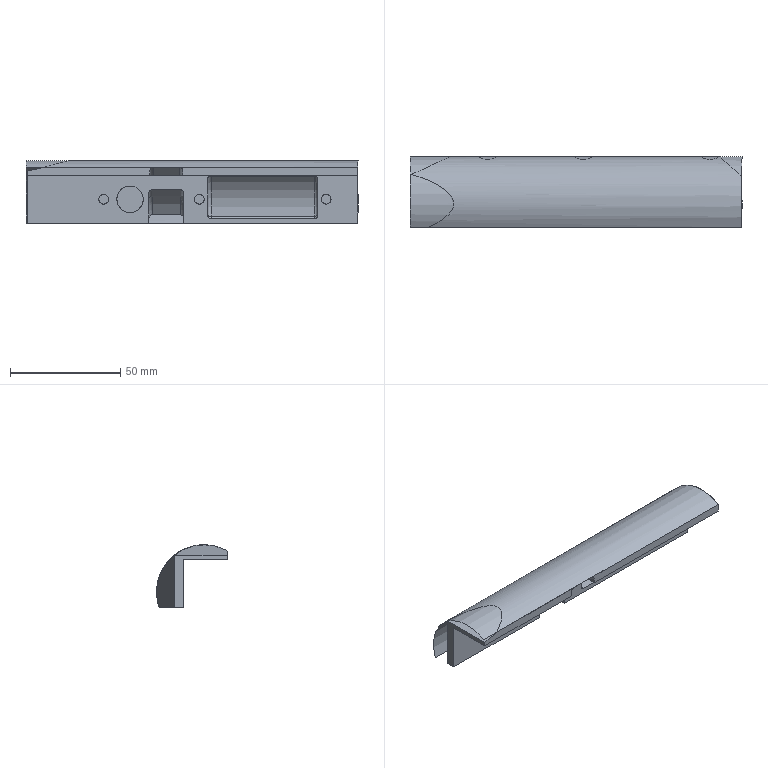NC program | Mastercam | posted with a generic post
Lines 1 to 31 of 52802:
%
:0001()
(MATERIAL - ALUMINUM MM - 2024)
(T24|100 FEM |H24)
(T9|10 FEM |H9|XY STOCK TO LEAVE - .15|Z STOCK TO LEAVE - 0.)
(T10|10 FEM |H10|XY STOCK TO LEAVE - -.02|Z STOCK TO LEAVE - 0.)
(T1|3 BM/BNOS |H1)
(T5|4 CHM |H5)
(T15|4.4 DR |H15)
(T4|4 FEM |H4|XY STOCK TO LEAVE - -.01|Z STOCK TO LEAVE - 0.)
(T17|6 BM/BNOS |H17)
(T18|10 BNOS |H18)
(T14|3.3 DR |H14)
N100 G21
N102 G0 G17 G40 G80 G90 G94 G98
N104 G0 G28 G91 Z0.
N106 G0 G28 X0. Y0.
(100 FEM |TOOL - 24|DIA. OFF. - 24|LEN. - 24|TOOL DIA. - 100.)
N108 T24 M6
N110 G0 G54 G90 X-180. Y0. C0. B0. S4000 M3
N112 G43 H24 Z25.
N114 Z1.
N116 G1 Z0. F600.
N118 X180. F1000.
N120 G0 Z25.
N122 M5
N124 G0 G28 G91 Z0.
N126 G28
N128 M01
N130 G0 G17 G40 G80 G90 G94 G98
N132 G0 G28 G91 Z0.